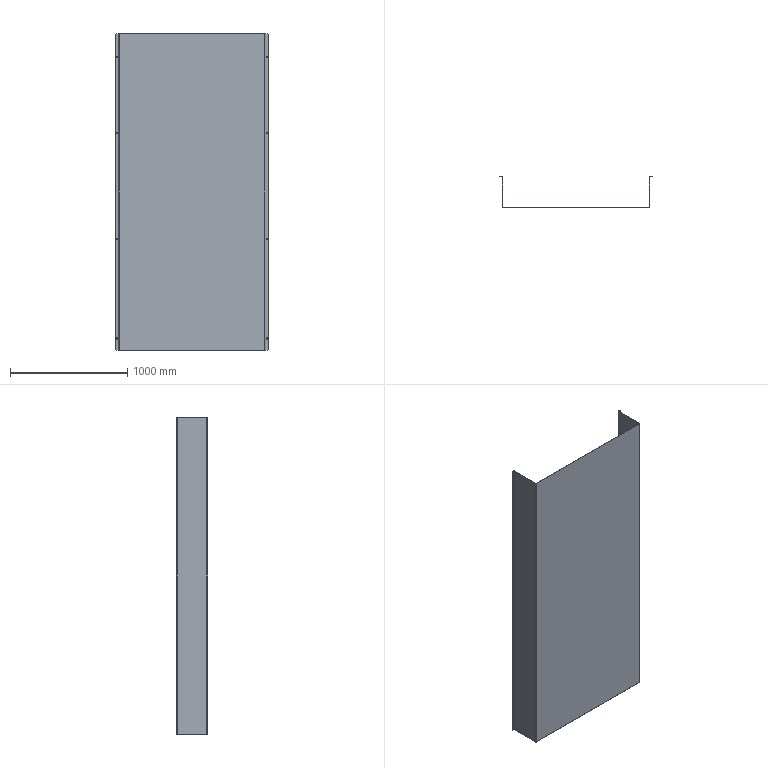Part | STEP file | VD-SYL0380DJ1006_1_2_1-1_STEP | 1 solid | 58 faces | box 1300 x 267 x 2700 mm | volume 14741994 mm3 | plane 34 | cylinder 24 | commonest cylinder face diameters 10.5 x16 6 x4 12 x4